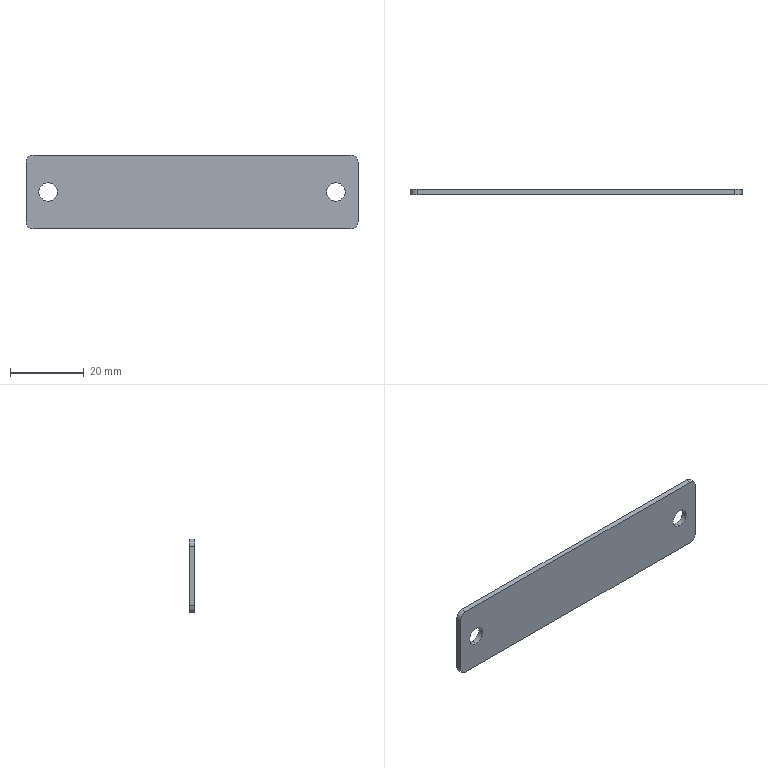Part | SolidWorks | features Extrusion 1, Fillet 1, ICE 1 | 1 solid | 14 faces | box 90 x 1.5 x 20 mm | volume 2636 mm3 | cylinder 8 | plane 6 | commonest cylinder face diameters 4 x4 5 x4
STEP:
#1=CARTESIAN_POINT('',(39.,0.,-2.5));
#2=VERTEX_POINT('',#1);
#3=CARTESIAN_POINT('',(39.,0.,2.5));
#4=VERTEX_POINT('',#3);
#5=CARTESIAN_POINT('',(39.,0.,0.));
#6=DIRECTION('',(0.,1.,0.));
#7=DIRECTION('',(0.,0.,1.));
#8=AXIS2_PLACEMENT_3D('',#5,#6,#7);
#9=CIRCLE('',#8,2.5);
#10=EDGE_CURVE('',#2,#4,#9,.T.);
#11=ORIENTED_EDGE('',*,*,#10,.F.);
#12=CARTESIAN_POINT('',(39.,1.5,-2.5));
#13=VERTEX_POINT('',#12);
#14=CARTESIAN_POINT('',(39.,0.,-2.5));
#15=DIRECTION('',(0.,1.,0.));
#16=VECTOR('',#15,1000.);
#17=LINE('',#14,#16);
#18=EDGE_CURVE('',#2,#13,#17,.T.);
#19=ORIENTED_EDGE('',*,*,#18,.T.);
#20=CARTESIAN_POINT('',(39.,1.5,2.5));
#21=VERTEX_POINT('',#20);
#22=CARTESIAN_POINT('',(39.,1.5,0.));
#23=DIRECTION('',(0.,1.,0.));
#24=DIRECTION('',(0.,0.,1.));
#25=AXIS2_PLACEMENT_3D('',#22,#23,#24);
#26=CIRCLE('',#25,2.5);
#27=EDGE_CURVE('',#13,#21,#26,.T.);
#28=ORIENTED_EDGE('',*,*,#27,.T.);
#29=CARTESIAN_POINT('',(39.,0.,2.5));
#30=DIRECTION('',(0.,1.,0.));
#31=VECTOR('',#30,1000.);
#32=LINE('',#29,#31);
#33=EDGE_CURVE('',#4,#21,#32,.T.);
#34=ORIENTED_EDGE('',*,*,#33,.F.);
#35=EDGE_LOOP('',(#11,#19,#28,#34));
#36=FACE_OUTER_BOUND('',#35,.T.);
#37=CARTESIAN_POINT('',(39.,0.,0.));
#38=DIRECTION('',(0.,1.,0.));
#39=DIRECTION('',(0.,0.,1.));
#40=AXIS2_PLACEMENT_3D('',#37,#38,#39);
#41=CYLINDRICAL_SURFACE('',#40,2.5);
#42=ADVANCED_FACE('',(#36),#41,.F.);
#43=CARTESIAN_POINT('',(-39.,0.,-2.5));
#44=VERTEX_POINT('',#43);
#45=CARTESIAN_POINT('',(-39.,0.,2.5));
#46=VERTEX_POINT('',#45);
#47=CARTESIAN_POINT('',(-39.,0.,0.));
#48=DIRECTION('',(0.,1.,0.));
#49=DIRECTION('',(0.,0.,1.));
#50=AXIS2_PLACEMENT_3D('',#47,#48,#49);
#51=CIRCLE('',#50,2.5);
#52=EDGE_CURVE('',#44,#46,#51,.T.);
#53=ORIENTED_EDGE('',*,*,#52,.F.);
#54=CARTESIAN_POINT('',(-39.,1.5,-2.5));
#55=VERTEX_POINT('',#54);
#56=CARTESIAN_POINT('',(-39.,0.,-2.5));
#57=DIRECTION('',(0.,1.,0.));
#58=VECTOR('',#57,1000.);
#59=LINE('',#56,#58);
#60=EDGE_CURVE('',#44,#55,#59,.T.);
#61=ORIENTED_EDGE('',*,*,#60,.T.);
#62=CARTESIAN_POINT('',(-39.,1.5,2.5));
#63=VERTEX_POINT('',#62);
#64=CARTESIAN_POINT('',(-39.,1.5,0.));
#65=DIRECTION('',(0.,1.,0.));
#66=DIRECTION('',(0.,0.,1.));
#67=AXIS2_PLACEMENT_3D('',#64,#65,#66);
#68=CIRCLE('',#67,2.5);
#69=EDGE_CURVE('',#55,#63,#68,.T.);
#70=ORIENTED_EDGE('',*,*,#69,.T.);
#71=CARTESIAN_POINT('',(-39.,0.,2.5));
#72=DIRECTION('',(0.,1.,0.));
#73=VECTOR('',#72,1000.);
#74=LINE('',#71,#73);
#75=EDGE_CURVE('',#46,#63,#74,.T.);
#76=ORIENTED_EDGE('',*,*,#75,.F.);
#77=EDGE_LOOP('',(#53,#61,#70,#76));
#78=FACE_OUTER_BOUND('',#77,.T.);
#79=CARTESIAN_POINT('',(-39.,0.,0.));
#80=DIRECTION('',(0.,1.,0.));
#81=DIRECTION('',(0.,0.,1.));
#82=AXIS2_PLACEMENT_3D('',#79,#80,#81);
#83=CYLINDRICAL_SURFACE('',#82,2.5);
#84=ADVANCED_FACE('',(#78),#83,.F.);
#85=CARTESIAN_POINT('',(45.,1.5,8.));
#86=VERTEX_POINT('',#85);
#87=CARTESIAN_POINT('',(45.,1.5,-8.));
#88=VERTEX_POINT('',#87);
#89=CARTESIAN_POINT('',(45.,1.5,10.));
#90=DIRECTION('',(0.,0.,-1.));
#91=VECTOR('',#90,1000.);
#92=LINE('',#89,#91);
#93=EDGE_CURVE('',#86,#88,#92,.T.);
#94=ORIENTED_EDGE('',*,*,#93,.F.);
#95=CARTESIAN_POINT('',(45.,0.,8.));
#96=VERTEX_POINT('',#95);
#97=CARTESIAN_POINT('',(45.,1.5,8.));
#98=DIRECTION('',(0.,-1.,0.));
#99=VECTOR('',#98,1000.);
#100=LINE('',#97,#99);
#101=EDGE_CURVE('',#86,#96,#100,.T.);
#102=ORIENTED_EDGE('',*,*,#101,.T.);
#103=CARTESIAN_POINT('',(45.,0.,-8.));
#104=VERTEX_POINT('',#103);
#105=CARTESIAN_POINT('',(45.,0.,10.));
#106=DIRECTION('',(0.,0.,-1.));
#107=VECTOR('',#106,1000.);
#108=LINE('',#105,#107);
#109=EDGE_CURVE('',#96,#104,#108,.T.);
#110=ORIENTED_EDGE('',*,*,#109,.T.);
#111=CARTESIAN_POINT('',(45.,1.5,-8.));
#112=DIRECTION('',(0.,1.,0.));
#113=VECTOR('',#112,1000.);
#114=LINE('',#111,#113);
#115=EDGE_CURVE('',#104,#88,#114,.T.);
#116=ORIENTED_EDGE('',*,*,#115,.T.);
#117=EDGE_LOOP('',(#94,#102,#110,#116));
#118=FACE_OUTER_BOUND('',#117,.T.);
#119=CARTESIAN_POINT('',(45.,1.5,10.));
#120=DIRECTION('',(-1.,0.,0.));
#121=DIRECTION('',(0.,0.,1.));
#122=AXIS2_PLACEMENT_3D('',#119,#120,#121);
#123=PLANE('',#122);
#124=ADVANCED_FACE('',(#118),#123,.F.);
#125=CARTESIAN_POINT('',(43.,1.5,-10.));
#126=VERTEX_POINT('',#125);
#127=CARTESIAN_POINT('',(-43.,1.5,-10.));
#128=VERTEX_POINT('',#127);
#129=CARTESIAN_POINT('',(-45.,1.5,-10.));
#130=DIRECTION('',(-1.,0.,0.));
#131=VECTOR('',#130,1000.);
#132=LINE('',#129,#131);
#133=EDGE_CURVE('',#126,#128,#132,.T.);
#134=ORIENTED_EDGE('',*,*,#133,.F.);
#135=CARTESIAN_POINT('',(43.,0.,-10.));
#136=VERTEX_POINT('',#135);
#137=CARTESIAN_POINT('',(43.,1.5,-10.));
#138=DIRECTION('',(0.,-1.,0.));
#139=VECTOR('',#138,1000.);
#140=LINE('',#137,#139);
#141=EDGE_CURVE('',#126,#136,#140,.T.);
#142=ORIENTED_EDGE('',*,*,#141,.T.);
#143=CARTESIAN_POINT('',(-43.,0.,-10.));
#144=VERTEX_POINT('',#143);
#145=CARTESIAN_POINT('',(-45.,0.,-10.));
#146=DIRECTION('',(-1.,0.,0.));
#147=VECTOR('',#146,1000.);
#148=LINE('',#145,#147);
#149=EDGE_CURVE('',#136,#144,#148,.T.);
#150=ORIENTED_EDGE('',*,*,#149,.T.);
#151=CARTESIAN_POINT('',(-43.,1.5,-10.));
#152=DIRECTION('',(0.,1.,0.));
#153=VECTOR('',#152,1000.);
#154=LINE('',#151,#153);
#155=EDGE_CURVE('',#144,#128,#154,.T.);
#156=ORIENTED_EDGE('',*,*,#155,.T.);
#157=EDGE_LOOP('',(#134,#142,#150,#156));
#158=FACE_OUTER_BOUND('',#157,.T.);
#159=CARTESIAN_POINT('',(-45.,1.5,-10.));
#160=DIRECTION('',(0.,0.,1.));
#161=DIRECTION('',(1.,0.,0.));
#162=AXIS2_PLACEMENT_3D('',#159,#160,#161);
#163=PLANE('',#162);
#164=ADVANCED_FACE('',(#158),#163,.F.);
#165=CARTESIAN_POINT('',(-45.,0.,-8.));
#166=VERTEX_POINT('',#165);
#167=CARTESIAN_POINT('',(-45.,0.,8.));
#168=VERTEX_POINT('',#167);
#169=CARTESIAN_POINT('',(-45.,0.,10.));
#170=DIRECTION('',(0.,0.,1.));
#171=VECTOR('',#170,1000.);
#172=LINE('',#169,#171);
#173=EDGE_CURVE('',#166,#168,#172,.T.);
#174=ORIENTED_EDGE('',*,*,#173,.T.);
#175=CARTESIAN_POINT('',(-45.,1.5,8.));
#176=VERTEX_POINT('',#175);
#177=CARTESIAN_POINT('',(-45.,1.5,8.));
#178=DIRECTION('',(0.,1.,0.));
#179=VECTOR('',#178,1000.);
#180=LINE('',#177,#179);
#181=EDGE_CURVE('',#168,#176,#180,.T.);
#182=ORIENTED_EDGE('',*,*,#181,.T.);
#183=CARTESIAN_POINT('',(-45.,1.5,-8.));
#184=VERTEX_POINT('',#183);
#185=CARTESIAN_POINT('',(-45.,1.5,10.));
#186=DIRECTION('',(0.,0.,1.));
#187=VECTOR('',#186,1000.);
#188=LINE('',#185,#187);
#189=EDGE_CURVE('',#184,#176,#188,.T.);
#190=ORIENTED_EDGE('',*,*,#189,.F.);
#191=CARTESIAN_POINT('',(-45.,1.5,-8.));
#192=DIRECTION('',(0.,-1.,0.));
#193=VECTOR('',#192,1000.);
#194=LINE('',#191,#193);
#195=EDGE_CURVE('',#184,#166,#194,.T.);
#196=ORIENTED_EDGE('',*,*,#195,.T.);
#197=EDGE_LOOP('',(#174,#182,#190,#196));
#198=FACE_OUTER_BOUND('',#197,.T.);
#199=CARTESIAN_POINT('',(-45.,1.5,10.));
#200=DIRECTION('',(1.,0.,0.));
#201=DIRECTION('',(0.,0.,-1.));
#202=AXIS2_PLACEMENT_3D('',#199,#200,#201);
#203=PLANE('',#202);
#204=ADVANCED_FACE('',(#198),#203,.F.);
#205=CARTESIAN_POINT('',(-43.,0.,10.));
#206=VERTEX_POINT('',#205);
#207=CARTESIAN_POINT('',(43.,0.,10.));
#208=VERTEX_POINT('',#207);
#209=CARTESIAN_POINT('',(-45.,0.,10.));
#210=DIRECTION('',(1.,0.,0.));
#211=VECTOR('',#210,1000.);
#212=LINE('',#209,#211);
#213=EDGE_CURVE('',#206,#208,#212,.T.);
#214=ORIENTED_EDGE('',*,*,#213,.T.);
#215=CARTESIAN_POINT('',(43.,1.5,10.));
#216=VERTEX_POINT('',#215);
#217=CARTESIAN_POINT('',(43.,1.5,10.));
#218=DIRECTION('',(0.,1.,0.));
#219=VECTOR('',#218,1000.);
#220=LINE('',#217,#219);
#221=EDGE_CURVE('',#208,#216,#220,.T.);
#222=ORIENTED_EDGE('',*,*,#221,.T.);
#223=CARTESIAN_POINT('',(-43.,1.5,10.));
#224=VERTEX_POINT('',#223);
#225=CARTESIAN_POINT('',(-45.,1.5,10.));
#226=DIRECTION('',(1.,0.,0.));
#227=VECTOR('',#226,1000.);
#228=LINE('',#225,#227);
#229=EDGE_CURVE('',#224,#216,#228,.T.);
#230=ORIENTED_EDGE('',*,*,#229,.F.);
#231=CARTESIAN_POINT('',(-43.,1.5,10.));
#232=DIRECTION('',(0.,-1.,0.));
#233=VECTOR('',#232,1000.);
#234=LINE('',#231,#233);
#235=EDGE_CURVE('',#224,#206,#234,.T.);
#236=ORIENTED_EDGE('',*,*,#235,.T.);
#237=EDGE_LOOP('',(#214,#222,#230,#236));
#238=FACE_OUTER_BOUND('',#237,.T.);
#239=CARTESIAN_POINT('',(-45.,1.5,10.));
#240=DIRECTION('',(0.,0.,-1.));
#241=DIRECTION('',(-1.,0.,0.));
#242=AXIS2_PLACEMENT_3D('',#239,#240,#241);
#243=PLANE('',#242);
#244=ADVANCED_FACE('',(#238),#243,.F.);
#245=CARTESIAN_POINT('',(39.,1.5,0.));
#246=DIRECTION('',(0.,1.,0.));
#247=DIRECTION('',(0.,0.,1.));
#248=AXIS2_PLACEMENT_3D('',#245,#246,#247);
#249=CIRCLE('',#248,2.5);
#250=EDGE_CURVE('',#21,#13,#249,.T.);
#251=ORIENTED_EDGE('',*,*,#250,.F.);
#252=ORIENTED_EDGE('',*,*,#27,.F.);
#253=EDGE_LOOP('',(#251,#252));
#254=FACE_BOUND('',#253,.T.);
#255=CARTESIAN_POINT('',(-39.,1.5,0.));
#256=DIRECTION('',(0.,1.,0.));
#257=DIRECTION('',(0.,0.,1.));
#258=AXIS2_PLACEMENT_3D('',#255,#256,#257);
#259=CIRCLE('',#258,2.5);
#260=EDGE_CURVE('',#63,#55,#259,.T.);
#261=ORIENTED_EDGE('',*,*,#260,.F.);
#262=ORIENTED_EDGE('',*,*,#69,.F.);
#263=EDGE_LOOP('',(#261,#262));
#264=FACE_BOUND('',#263,.T.);
#265=ORIENTED_EDGE('',*,*,#229,.T.);
#266=CARTESIAN_POINT('',(43.,1.5,8.));
#267=DIRECTION('',(0.,1.,0.));
#268=DIRECTION('',(0.,0.,-1.));
#269=AXIS2_PLACEMENT_3D('',#266,#267,#268);
#270=CIRCLE('',#269,2.);
#271=EDGE_CURVE('',#216,#86,#270,.T.);
#272=ORIENTED_EDGE('',*,*,#271,.T.);
#273=ORIENTED_EDGE('',*,*,#93,.T.);
#274=CARTESIAN_POINT('',(43.,1.5,-8.));
#275=DIRECTION('',(0.,1.,0.));
#276=DIRECTION('',(0.,0.,-1.));
#277=AXIS2_PLACEMENT_3D('',#274,#275,#276);
#278=CIRCLE('',#277,2.);
#279=EDGE_CURVE('',#88,#126,#278,.T.);
#280=ORIENTED_EDGE('',*,*,#279,.T.);
#281=ORIENTED_EDGE('',*,*,#133,.T.);
#282=CARTESIAN_POINT('',(-43.,1.5,-8.));
#283=DIRECTION('',(0.,1.,0.));
#284=DIRECTION('',(0.,0.,-1.));
#285=AXIS2_PLACEMENT_3D('',#282,#283,#284);
#286=CIRCLE('',#285,2.);
#287=EDGE_CURVE('',#128,#184,#286,.T.);
#288=ORIENTED_EDGE('',*,*,#287,.T.);
#289=ORIENTED_EDGE('',*,*,#189,.T.);
#290=CARTESIAN_POINT('',(-43.,1.5,8.));
#291=DIRECTION('',(0.,1.,0.));
#292=DIRECTION('',(0.,0.,-1.));
#293=AXIS2_PLACEMENT_3D('',#290,#291,#292);
#294=CIRCLE('',#293,2.);
#295=EDGE_CURVE('',#176,#224,#294,.T.);
#296=ORIENTED_EDGE('',*,*,#295,.T.);
#297=EDGE_LOOP('',(#265,#272,#273,#280,#281,#288,#289,#296));
#298=FACE_OUTER_BOUND('',#297,.T.);
#299=CARTESIAN_POINT('',(45.,1.5,-10.));
#300=DIRECTION('',(0.,-1.,0.));
#301=DIRECTION('',(0.,0.,-1.));
#302=AXIS2_PLACEMENT_3D('',#299,#300,#301);
#303=PLANE('',#302);
#304=ADVANCED_FACE('',(#254,#264,#298),#303,.F.);
#305=CARTESIAN_POINT('',(39.,0.,0.));
#306=DIRECTION('',(0.,1.,0.));
#307=DIRECTION('',(0.,0.,1.));
#308=AXIS2_PLACEMENT_3D('',#305,#306,#307);
#309=CIRCLE('',#308,2.5);
#310=EDGE_CURVE('',#4,#2,#309,.T.);
#311=ORIENTED_EDGE('',*,*,#310,.T.);
#312=ORIENTED_EDGE('',*,*,#10,.T.);
#313=EDGE_LOOP('',(#311,#312));
#314=FACE_BOUND('',#313,.T.);
#315=CARTESIAN_POINT('',(-39.,0.,0.));
#316=DIRECTION('',(0.,1.,0.));
#317=DIRECTION('',(0.,0.,1.));
#318=AXIS2_PLACEMENT_3D('',#315,#316,#317);
#319=CIRCLE('',#318,2.5);
#320=EDGE_CURVE('',#46,#44,#319,.T.);
#321=ORIENTED_EDGE('',*,*,#320,.T.);
#322=ORIENTED_EDGE('',*,*,#52,.T.);
#323=EDGE_LOOP('',(#321,#322));
#324=FACE_BOUND('',#323,.T.);
#325=ORIENTED_EDGE('',*,*,#109,.F.);
#326=CARTESIAN_POINT('',(43.,0.,8.));
#327=DIRECTION('',(0.,-1.,0.));
#328=DIRECTION('',(0.,0.,-1.));
#329=AXIS2_PLACEMENT_3D('',#326,#327,#328);
#330=CIRCLE('',#329,2.);
#331=EDGE_CURVE('',#96,#208,#330,.T.);
#332=ORIENTED_EDGE('',*,*,#331,.T.);
#333=ORIENTED_EDGE('',*,*,#213,.F.);
#334=CARTESIAN_POINT('',(-43.,0.,8.));
#335=DIRECTION('',(0.,-1.,0.));
#336=DIRECTION('',(0.,0.,-1.));
#337=AXIS2_PLACEMENT_3D('',#334,#335,#336);
#338=CIRCLE('',#337,2.);
#339=EDGE_CURVE('',#206,#168,#338,.T.);
#340=ORIENTED_EDGE('',*,*,#339,.T.);
#341=ORIENTED_EDGE('',*,*,#173,.F.);
#342=CARTESIAN_POINT('',(-43.,0.,-8.));
#343=DIRECTION('',(0.,-1.,0.));
#344=DIRECTION('',(0.,0.,-1.));
#345=AXIS2_PLACEMENT_3D('',#342,#343,#344);
#346=CIRCLE('',#345,2.);
#347=EDGE_CURVE('',#166,#144,#346,.T.);
#348=ORIENTED_EDGE('',*,*,#347,.T.);
#349=ORIENTED_EDGE('',*,*,#149,.F.);
#350=CARTESIAN_POINT('',(43.,0.,-8.));
#351=DIRECTION('',(0.,-1.,0.));
#352=DIRECTION('',(0.,0.,-1.));
#353=AXIS2_PLACEMENT_3D('',#350,#351,#352);
#354=CIRCLE('',#353,2.);
#355=EDGE_CURVE('',#136,#104,#354,.T.);
#356=ORIENTED_EDGE('',*,*,#355,.T.);
#357=EDGE_LOOP('',(#325,#332,#333,#340,#341,#348,#349,#356));
#358=FACE_OUTER_BOUND('',#357,.T.);
#359=CARTESIAN_POINT('',(45.,0.,-10.));
#360=DIRECTION('',(0.,-1.,0.));
#361=DIRECTION('',(0.,0.,-1.));
#362=AXIS2_PLACEMENT_3D('',#359,#360,#361);
#363=PLANE('',#362);
#364=ADVANCED_FACE('',(#314,#324,#358),#363,.T.);
#365=ORIENTED_EDGE('',*,*,#60,.F.);
#366=ORIENTED_EDGE('',*,*,#320,.F.);
#367=ORIENTED_EDGE('',*,*,#75,.T.);
#368=ORIENTED_EDGE('',*,*,#260,.T.);
#369=EDGE_LOOP('',(#365,#366,#367,#368));
#370=FACE_OUTER_BOUND('',#369,.T.);
#371=CARTESIAN_POINT('',(-39.,0.,0.));
#372=DIRECTION('',(0.,1.,0.));
#373=DIRECTION('',(0.,0.,1.));
#374=AXIS2_PLACEMENT_3D('',#371,#372,#373);
#375=CYLINDRICAL_SURFACE('',#374,2.5);
#376=ADVANCED_FACE('',(#370),#375,.F.);
#377=ORIENTED_EDGE('',*,*,#18,.F.);
#378=ORIENTED_EDGE('',*,*,#310,.F.);
#379=ORIENTED_EDGE('',*,*,#33,.T.);
#380=ORIENTED_EDGE('',*,*,#250,.T.);
#381=EDGE_LOOP('',(#377,#378,#379,#380));
#382=FACE_OUTER_BOUND('',#381,.T.);
#383=CARTESIAN_POINT('',(39.,0.,0.));
#384=DIRECTION('',(0.,1.,0.));
#385=DIRECTION('',(0.,0.,1.));
#386=AXIS2_PLACEMENT_3D('',#383,#384,#385);
#387=CYLINDRICAL_SURFACE('',#386,2.5);
#388=ADVANCED_FACE('',(#382),#387,.F.);
#389=ORIENTED_EDGE('',*,*,#271,.F.);
#390=ORIENTED_EDGE('',*,*,#221,.F.);
#391=ORIENTED_EDGE('',*,*,#331,.F.);
#392=ORIENTED_EDGE('',*,*,#101,.F.);
#393=EDGE_LOOP('',(#389,#390,#391,#392));
#394=FACE_OUTER_BOUND('',#393,.T.);
#395=CARTESIAN_POINT('',(43.,1.5,8.));
#396=DIRECTION('',(0.,-1.,0.));
#397=DIRECTION('',(0.,0.,-1.));
#398=AXIS2_PLACEMENT_3D('',#395,#396,#397);
#399=CYLINDRICAL_SURFACE('',#398,2.);
#400=ADVANCED_FACE('',(#394),#399,.T.);
#401=ORIENTED_EDGE('',*,*,#279,.F.);
#402=ORIENTED_EDGE('',*,*,#115,.F.);
#403=ORIENTED_EDGE('',*,*,#355,.F.);
#404=ORIENTED_EDGE('',*,*,#141,.F.);
#405=EDGE_LOOP('',(#401,#402,#403,#404));
#406=FACE_OUTER_BOUND('',#405,.T.);
#407=CARTESIAN_POINT('',(43.,1.5,-8.));
#408=DIRECTION('',(0.,-1.,0.));
#409=DIRECTION('',(0.,0.,-1.));
#410=AXIS2_PLACEMENT_3D('',#407,#408,#409);
#411=CYLINDRICAL_SURFACE('',#410,2.);
#412=ADVANCED_FACE('',(#406),#411,.T.);
#413=ORIENTED_EDGE('',*,*,#295,.F.);
#414=ORIENTED_EDGE('',*,*,#181,.F.);
#415=ORIENTED_EDGE('',*,*,#339,.F.);
#416=ORIENTED_EDGE('',*,*,#235,.F.);
#417=EDGE_LOOP('',(#413,#414,#415,#416));
#418=FACE_OUTER_BOUND('',#417,.T.);
#419=CARTESIAN_POINT('',(-43.,1.5,8.));
#420=DIRECTION('',(0.,-1.,0.));
#421=DIRECTION('',(0.,0.,-1.));
#422=AXIS2_PLACEMENT_3D('',#419,#420,#421);
#423=CYLINDRICAL_SURFACE('',#422,2.);
#424=ADVANCED_FACE('',(#418),#423,.T.);
#425=ORIENTED_EDGE('',*,*,#287,.F.);
#426=ORIENTED_EDGE('',*,*,#155,.F.);
#427=ORIENTED_EDGE('',*,*,#347,.F.);
#428=ORIENTED_EDGE('',*,*,#195,.F.);
#429=EDGE_LOOP('',(#425,#426,#427,#428));
#430=FACE_OUTER_BOUND('',#429,.T.);
#431=CARTESIAN_POINT('',(-43.,1.5,-8.));
#432=DIRECTION('',(0.,-1.,0.));
#433=DIRECTION('',(0.,0.,-1.));
#434=AXIS2_PLACEMENT_3D('',#431,#432,#433);
#435=CYLINDRICAL_SURFACE('',#434,2.);
#436=ADVANCED_FACE('',(#430),#435,.T.);
#437=CLOSED_SHELL('',(#42,#84,#124,#164,#204,#244,#304,#364,#376,#388,#400,#412,#424,#436));
#438=MANIFOLD_SOLID_BREP('',#437);
#439=CARTESIAN_POINT('',(0.,0.,0.));
#440=DIRECTION('',(0.,0.,1.));
#441=DIRECTION('',(1.,0.,0.));
#442=AXIS2_PLACEMENT_3D('',#439,#440,#441);
#443=(LENGTH_UNIT()NAMED_UNIT(*)SI_UNIT(.MILLI.,.METRE.));
#444=UNCERTAINTY_MEASURE_WITH_UNIT(LENGTH_MEASURE(0.00001),#443,'','');
#445=(NAMED_UNIT(*)PLANE_ANGLE_UNIT()SI_UNIT($,.RADIAN.));
#446=(NAMED_UNIT(*)SI_UNIT($,.STERADIAN.)SOLID_ANGLE_UNIT());
#447=(GEOMETRIC_REPRESENTATION_CONTEXT(3)GLOBAL_UNCERTAINTY_ASSIGNED_CONTEXT((#444))GLOBAL_UNIT_ASSIGNED_CONTEXT((#443,#445,#446))REPRESENTATION_CONTEXT('',''));
#448=ADVANCED_BREP_SHAPE_REPRESENTATION('',(#438,#442),#447);